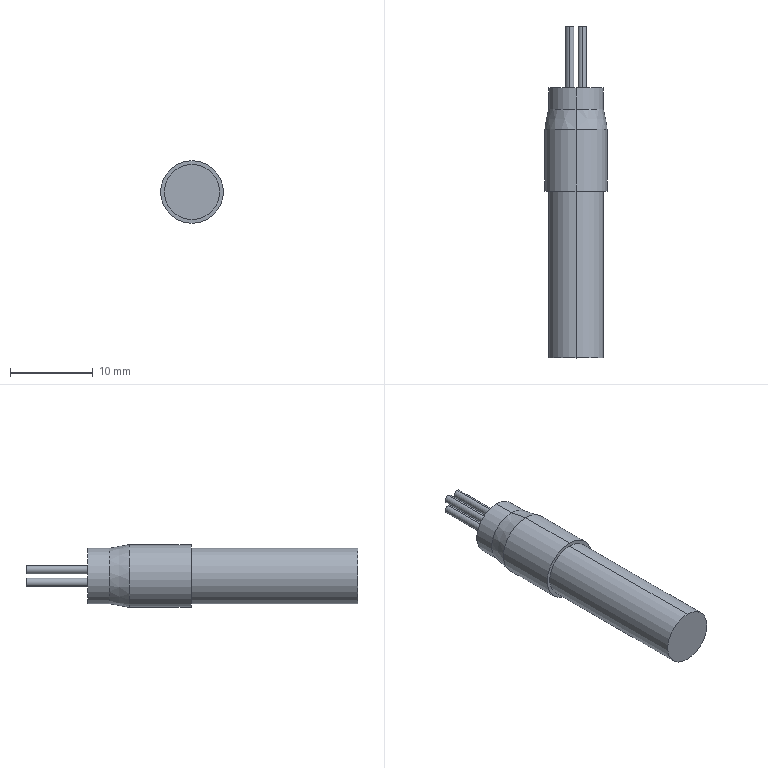Part | SolidWorks | features BaseBody 1 | 1 solid | 23 faces | box 7.6 x 40.2 x 7.6 mm | volume 1264 mm3 | cylinder 14 | plane 7 | cone 2 | commonest cylinder face diameters 1 x8 6.7 x4 7.6 x2
STEP:
#1=CARTESIAN_POINT('',(0.,72.3,3.35));
#2=VERTEX_POINT('',#1);
#3=CARTESIAN_POINT('',(0.,72.3,-3.35));
#4=VERTEX_POINT('',#3);
#5=CARTESIAN_POINT('',(0.,72.3,0.));
#6=DIRECTION('',(0.,1.,0.));
#7=DIRECTION('',(0.,0.,1.));
#8=AXIS2_PLACEMENT_3D('',#5,#6,#7);
#9=CIRCLE('',#8,3.35);
#10=EDGE_CURVE('',#2,#4,#9,.T.);
#11=ORIENTED_EDGE('',*,*,#10,.T.);
#12=CARTESIAN_POINT('',(0.,92.5,-3.35));
#13=VERTEX_POINT('',#12);
#14=CARTESIAN_POINT('',(0.,95.,-3.35));
#15=DIRECTION('',(0.,1.,0.));
#16=VECTOR('',#15,1000.);
#17=LINE('',#14,#16);
#18=EDGE_CURVE('',#4,#13,#17,.T.);
#19=ORIENTED_EDGE('',*,*,#18,.T.);
#20=CARTESIAN_POINT('',(0.,92.5,3.35));
#21=VERTEX_POINT('',#20);
#22=CARTESIAN_POINT('',(0.,92.5,0.));
#23=DIRECTION('',(0.,-1.,0.));
#24=DIRECTION('',(0.,0.,1.));
#25=AXIS2_PLACEMENT_3D('',#22,#23,#24);
#26=CIRCLE('',#25,3.35);
#27=EDGE_CURVE('',#13,#21,#26,.T.);
#28=ORIENTED_EDGE('',*,*,#27,.T.);
#29=CARTESIAN_POINT('',(0.,95.,3.35));
#30=DIRECTION('',(0.,1.,0.));
#31=VECTOR('',#30,1000.);
#32=LINE('',#29,#31);
#33=EDGE_CURVE('',#2,#21,#32,.T.);
#34=ORIENTED_EDGE('',*,*,#33,.F.);
#35=EDGE_LOOP('',(#11,#19,#28,#34));
#36=FACE_OUTER_BOUND('',#35,.T.);
#37=CARTESIAN_POINT('',(0.,95.,0.));
#38=DIRECTION('',(0.,1.,0.));
#39=DIRECTION('',(0.,0.,1.));
#40=AXIS2_PLACEMENT_3D('',#37,#38,#39);
#41=CYLINDRICAL_SURFACE('',#40,3.35);
#42=ADVANCED_FACE('',(#36),#41,.T.);
#43=CARTESIAN_POINT('',(0.,92.5,3.8));
#44=VERTEX_POINT('',#43);
#45=CARTESIAN_POINT('',(0.,92.5,-3.8));
#46=VERTEX_POINT('',#45);
#47=CARTESIAN_POINT('',(0.,92.5,0.));
#48=DIRECTION('',(0.,1.,0.));
#49=DIRECTION('',(0.,0.,1.));
#50=AXIS2_PLACEMENT_3D('',#47,#48,#49);
#51=CIRCLE('',#50,3.8);
#52=EDGE_CURVE('',#44,#46,#51,.T.);
#53=ORIENTED_EDGE('',*,*,#52,.T.);
#54=CARTESIAN_POINT('',(0.,100.,-3.8));
#55=VERTEX_POINT('',#54);
#56=CARTESIAN_POINT('',(0.,92.5,-3.8));
#57=DIRECTION('',(0.,1.,0.));
#58=VECTOR('',#57,1000.);
#59=LINE('',#56,#58);
#60=EDGE_CURVE('',#46,#55,#59,.T.);
#61=ORIENTED_EDGE('',*,*,#60,.T.);
#62=CARTESIAN_POINT('',(0.,100.,3.8));
#63=VERTEX_POINT('',#62);
#64=CARTESIAN_POINT('',(0.,100.,0.));
#65=DIRECTION('',(0.,-1.,0.));
#66=DIRECTION('',(0.,0.,1.));
#67=AXIS2_PLACEMENT_3D('',#64,#65,#66);
#68=CIRCLE('',#67,3.8);
#69=EDGE_CURVE('',#55,#63,#68,.T.);
#70=ORIENTED_EDGE('',*,*,#69,.T.);
#71=CARTESIAN_POINT('',(0.,92.5,3.8));
#72=DIRECTION('',(0.,1.,0.));
#73=VECTOR('',#72,1000.);
#74=LINE('',#71,#73);
#75=EDGE_CURVE('',#44,#63,#74,.T.);
#76=ORIENTED_EDGE('',*,*,#75,.F.);
#77=EDGE_LOOP('',(#53,#61,#70,#76));
#78=FACE_OUTER_BOUND('',#77,.T.);
#79=CARTESIAN_POINT('',(0.,92.5,0.));
#80=DIRECTION('',(0.,1.,0.));
#81=DIRECTION('',(0.,0.,1.));
#82=AXIS2_PLACEMENT_3D('',#79,#80,#81);
#83=CYLINDRICAL_SURFACE('',#82,3.8);
#84=ADVANCED_FACE('',(#78),#83,.T.);
#85=CARTESIAN_POINT('',(0.,102.426,-3.35));
#86=VERTEX_POINT('',#85);
#87=CARTESIAN_POINT('',(0.,102.426,3.35));
#88=VERTEX_POINT('',#87);
#89=CARTESIAN_POINT('',(0.,102.426,0.));
#90=DIRECTION('',(0.,-1.,0.));
#91=DIRECTION('',(0.,0.,-1.));
#92=AXIS2_PLACEMENT_3D('',#89,#90,#91);
#93=CIRCLE('',#92,3.35);
#94=EDGE_CURVE('',#86,#88,#93,.T.);
#95=ORIENTED_EDGE('',*,*,#94,.T.);
#96=CARTESIAN_POINT('',(0.,100.,3.8));
#97=DIRECTION('',(0.,-0.9832,0.1824));
#98=VECTOR('',#97,1000.);
#99=LINE('',#96,#98);
#100=EDGE_CURVE('',#88,#63,#99,.T.);
#101=ORIENTED_EDGE('',*,*,#100,.T.);
#102=ORIENTED_EDGE('',*,*,#69,.F.);
#103=CARTESIAN_POINT('',(0.,100.,-3.8));
#104=DIRECTION('',(0.,-0.9832,-0.1824));
#105=VECTOR('',#104,1000.);
#106=LINE('',#103,#105);
#107=EDGE_CURVE('',#86,#55,#106,.T.);
#108=ORIENTED_EDGE('',*,*,#107,.F.);
#109=EDGE_LOOP('',(#95,#101,#102,#108));
#110=FACE_OUTER_BOUND('',#109,.T.);
#111=CARTESIAN_POINT('',(0.,100.,0.));
#112=DIRECTION('',(0.,-1.,0.));
#113=DIRECTION('',(0.,0.,-1.));
#114=AXIS2_PLACEMENT_3D('',#111,#112,#113);
#115=CONICAL_SURFACE('',#114,3.8,0.1834);
#116=ADVANCED_FACE('',(#110),#115,.T.);
#117=ORIENTED_EDGE('',*,*,#94,.F.);
#118=CARTESIAN_POINT('',(0.,105.,-3.35));
#119=VERTEX_POINT('',#118);
#120=CARTESIAN_POINT('',(0.,92.5,-3.35));
#121=DIRECTION('',(0.,1.,0.));
#122=VECTOR('',#121,1000.);
#123=LINE('',#120,#122);
#124=EDGE_CURVE('',#86,#119,#123,.T.);
#125=ORIENTED_EDGE('',*,*,#124,.T.);
#126=CARTESIAN_POINT('',(0.,105.,3.35));
#127=VERTEX_POINT('',#126);
#128=CARTESIAN_POINT('',(0.,105.,0.));
#129=DIRECTION('',(0.,-1.,0.));
#130=DIRECTION('',(0.,0.,1.));
#131=AXIS2_PLACEMENT_3D('',#128,#129,#130);
#132=CIRCLE('',#131,3.35);
#133=EDGE_CURVE('',#119,#127,#132,.T.);
#134=ORIENTED_EDGE('',*,*,#133,.T.);
#135=CARTESIAN_POINT('',(0.,92.5,3.35));
#136=DIRECTION('',(0.,1.,0.));
#137=VECTOR('',#136,1000.);
#138=LINE('',#135,#137);
#139=EDGE_CURVE('',#88,#127,#138,.T.);
#140=ORIENTED_EDGE('',*,*,#139,.F.);
#141=EDGE_LOOP('',(#117,#125,#134,#140));
#142=FACE_OUTER_BOUND('',#141,.T.);
#143=CARTESIAN_POINT('',(0.,92.5,0.));
#144=DIRECTION('',(0.,1.,0.));
#145=DIRECTION('',(0.,0.,1.));
#146=AXIS2_PLACEMENT_3D('',#143,#144,#145);
#147=CYLINDRICAL_SURFACE('',#146,3.35);
#148=ADVANCED_FACE('',(#142),#147,.T.);
#149=CARTESIAN_POINT('',(0.75,105.,-0.25));
#150=VERTEX_POINT('',#149);
#151=CARTESIAN_POINT('',(0.75,105.,-1.25));
#152=VERTEX_POINT('',#151);
#153=CARTESIAN_POINT('',(0.75,105.,-0.75));
#154=DIRECTION('',(0.,1.,0.));
#155=DIRECTION('',(0.,0.,1.));
#156=AXIS2_PLACEMENT_3D('',#153,#154,#155);
#157=CIRCLE('',#156,0.5);
#158=EDGE_CURVE('',#150,#152,#157,.T.);
#159=ORIENTED_EDGE('',*,*,#158,.T.);
#160=CARTESIAN_POINT('',(0.75,112.5,-1.25));
#161=VERTEX_POINT('',#160);
#162=CARTESIAN_POINT('',(0.75,112.5,-1.25));
#163=DIRECTION('',(0.,1.,0.));
#164=VECTOR('',#163,1000.);
#165=LINE('',#162,#164);
#166=EDGE_CURVE('',#152,#161,#165,.T.);
#167=ORIENTED_EDGE('',*,*,#166,.T.);
#168=CARTESIAN_POINT('',(0.75,112.5,-0.25));
#169=VERTEX_POINT('',#168);
#170=CARTESIAN_POINT('',(0.75,112.5,-0.75));
#171=DIRECTION('',(0.,-1.,0.));
#172=DIRECTION('',(0.,0.,1.));
#173=AXIS2_PLACEMENT_3D('',#170,#171,#172);
#174=CIRCLE('',#173,0.5);
#175=EDGE_CURVE('',#161,#169,#174,.T.);
#176=ORIENTED_EDGE('',*,*,#175,.T.);
#177=CARTESIAN_POINT('',(0.75,112.5,-0.25));
#178=DIRECTION('',(0.,1.,0.));
#179=VECTOR('',#178,1000.);
#180=LINE('',#177,#179);
#181=EDGE_CURVE('',#150,#169,#180,.T.);
#182=ORIENTED_EDGE('',*,*,#181,.F.);
#183=EDGE_LOOP('',(#159,#167,#176,#182));
#184=FACE_OUTER_BOUND('',#183,.T.);
#185=CARTESIAN_POINT('',(0.75,112.5,-0.75));
#186=DIRECTION('',(0.,1.,0.));
#187=DIRECTION('',(0.,0.,1.));
#188=AXIS2_PLACEMENT_3D('',#185,#186,#187);
#189=CYLINDRICAL_SURFACE('',#188,0.5);
#190=ADVANCED_FACE('',(#184),#189,.T.);
#191=CARTESIAN_POINT('',(-0.75,105.,-0.25));
#192=VERTEX_POINT('',#191);
#193=CARTESIAN_POINT('',(-0.75,105.,-1.25));
#194=VERTEX_POINT('',#193);
#195=CARTESIAN_POINT('',(-0.75,105.,-0.75));
#196=DIRECTION('',(0.,1.,0.));
#197=DIRECTION('',(0.,0.,1.));
#198=AXIS2_PLACEMENT_3D('',#195,#196,#197);
#199=CIRCLE('',#198,0.5);
#200=EDGE_CURVE('',#192,#194,#199,.T.);
#201=ORIENTED_EDGE('',*,*,#200,.T.);
#202=CARTESIAN_POINT('',(-0.75,112.5,-1.25));
#203=VERTEX_POINT('',#202);
#204=CARTESIAN_POINT('',(-0.75,112.5,-1.25));
#205=DIRECTION('',(0.,1.,0.));
#206=VECTOR('',#205,1000.);
#207=LINE('',#204,#206);
#208=EDGE_CURVE('',#194,#203,#207,.T.);
#209=ORIENTED_EDGE('',*,*,#208,.T.);
#210=CARTESIAN_POINT('',(-0.75,112.5,-0.25));
#211=VERTEX_POINT('',#210);
#212=CARTESIAN_POINT('',(-0.75,112.5,-0.75));
#213=DIRECTION('',(0.,-1.,0.));
#214=DIRECTION('',(0.,0.,1.));
#215=AXIS2_PLACEMENT_3D('',#212,#213,#214);
#216=CIRCLE('',#215,0.5);
#217=EDGE_CURVE('',#203,#211,#216,.T.);
#218=ORIENTED_EDGE('',*,*,#217,.T.);
#219=CARTESIAN_POINT('',(-0.75,112.5,-0.25));
#220=DIRECTION('',(0.,1.,0.));
#221=VECTOR('',#220,1000.);
#222=LINE('',#219,#221);
#223=EDGE_CURVE('',#192,#211,#222,.T.);
#224=ORIENTED_EDGE('',*,*,#223,.F.);
#225=EDGE_LOOP('',(#201,#209,#218,#224));
#226=FACE_OUTER_BOUND('',#225,.T.);
#227=CARTESIAN_POINT('',(-0.75,112.5,-0.75));
#228=DIRECTION('',(0.,1.,0.));
#229=DIRECTION('',(0.,0.,1.));
#230=AXIS2_PLACEMENT_3D('',#227,#228,#229);
#231=CYLINDRICAL_SURFACE('',#230,0.5);
#232=ADVANCED_FACE('',(#226),#231,.T.);
#233=CARTESIAN_POINT('',(-0.75,105.,1.25));
#234=VERTEX_POINT('',#233);
#235=CARTESIAN_POINT('',(-0.75,105.,0.25));
#236=VERTEX_POINT('',#235);
#237=CARTESIAN_POINT('',(-0.75,105.,0.75));
#238=DIRECTION('',(0.,1.,0.));
#239=DIRECTION('',(0.,0.,1.));
#240=AXIS2_PLACEMENT_3D('',#237,#238,#239);
#241=CIRCLE('',#240,0.5);
#242=EDGE_CURVE('',#234,#236,#241,.T.);
#243=ORIENTED_EDGE('',*,*,#242,.T.);
#244=CARTESIAN_POINT('',(-0.75,112.5,0.25));
#245=VERTEX_POINT('',#244);
#246=CARTESIAN_POINT('',(-0.75,112.5,0.25));
#247=DIRECTION('',(0.,1.,0.));
#248=VECTOR('',#247,1000.);
#249=LINE('',#246,#248);
#250=EDGE_CURVE('',#236,#245,#249,.T.);
#251=ORIENTED_EDGE('',*,*,#250,.T.);
#252=CARTESIAN_POINT('',(-0.75,112.5,1.25));
#253=VERTEX_POINT('',#252);
#254=CARTESIAN_POINT('',(-0.75,112.5,0.75));
#255=DIRECTION('',(0.,-1.,0.));
#256=DIRECTION('',(0.,0.,1.));
#257=AXIS2_PLACEMENT_3D('',#254,#255,#256);
#258=CIRCLE('',#257,0.5);
#259=EDGE_CURVE('',#245,#253,#258,.T.);
#260=ORIENTED_EDGE('',*,*,#259,.T.);
#261=CARTESIAN_POINT('',(-0.75,112.5,1.25));
#262=DIRECTION('',(0.,1.,0.));
#263=VECTOR('',#262,1000.);
#264=LINE('',#261,#263);
#265=EDGE_CURVE('',#234,#253,#264,.T.);
#266=ORIENTED_EDGE('',*,*,#265,.F.);
#267=EDGE_LOOP('',(#243,#251,#260,#266));
#268=FACE_OUTER_BOUND('',#267,.T.);
#269=CARTESIAN_POINT('',(-0.75,112.5,0.75));
#270=DIRECTION('',(0.,1.,0.));
#271=DIRECTION('',(0.,0.,1.));
#272=AXIS2_PLACEMENT_3D('',#269,#270,#271);
#273=CYLINDRICAL_SURFACE('',#272,0.5);
#274=ADVANCED_FACE('',(#268),#273,.T.);
#275=CARTESIAN_POINT('',(0.75,105.,1.25));
#276=VERTEX_POINT('',#275);
#277=CARTESIAN_POINT('',(0.75,105.,0.25));
#278=VERTEX_POINT('',#277);
#279=CARTESIAN_POINT('',(0.75,105.,0.75));
#280=DIRECTION('',(0.,1.,0.));
#281=DIRECTION('',(0.,0.,1.));
#282=AXIS2_PLACEMENT_3D('',#279,#280,#281);
#283=CIRCLE('',#282,0.5);
#284=EDGE_CURVE('',#276,#278,#283,.T.);
#285=ORIENTED_EDGE('',*,*,#284,.T.);
#286=CARTESIAN_POINT('',(0.75,112.5,0.25));
#287=VERTEX_POINT('',#286);
#288=CARTESIAN_POINT('',(0.75,112.5,0.25));
#289=DIRECTION('',(0.,1.,0.));
#290=VECTOR('',#289,1000.);
#291=LINE('',#288,#290);
#292=EDGE_CURVE('',#278,#287,#291,.T.);
#293=ORIENTED_EDGE('',*,*,#292,.T.);
#294=CARTESIAN_POINT('',(0.75,112.5,1.25));
#295=VERTEX_POINT('',#294);
#296=CARTESIAN_POINT('',(0.75,112.5,0.75));
#297=DIRECTION('',(0.,-1.,0.));
#298=DIRECTION('',(0.,0.,1.));
#299=AXIS2_PLACEMENT_3D('',#296,#297,#298);
#300=CIRCLE('',#299,0.5);
#301=EDGE_CURVE('',#287,#295,#300,.T.);
#302=ORIENTED_EDGE('',*,*,#301,.T.);
#303=CARTESIAN_POINT('',(0.75,112.5,1.25));
#304=DIRECTION('',(0.,1.,0.));
#305=VECTOR('',#304,1000.);
#306=LINE('',#303,#305);
#307=EDGE_CURVE('',#276,#295,#306,.T.);
#308=ORIENTED_EDGE('',*,*,#307,.F.);
#309=EDGE_LOOP('',(#285,#293,#302,#308));
#310=FACE_OUTER_BOUND('',#309,.T.);
#311=CARTESIAN_POINT('',(0.75,112.5,0.75));
#312=DIRECTION('',(0.,1.,0.));
#313=DIRECTION('',(0.,0.,1.));
#314=AXIS2_PLACEMENT_3D('',#311,#312,#313);
#315=CYLINDRICAL_SURFACE('',#314,0.5);
#316=ADVANCED_FACE('',(#310),#315,.T.);
#317=ORIENTED_EDGE('',*,*,#18,.F.);
#318=CARTESIAN_POINT('',(0.,72.3,0.));
#319=DIRECTION('',(0.,1.,0.));
#320=DIRECTION('',(0.,0.,1.));
#321=AXIS2_PLACEMENT_3D('',#318,#319,#320);
#322=CIRCLE('',#321,3.35);
#323=EDGE_CURVE('',#4,#2,#322,.T.);
#324=ORIENTED_EDGE('',*,*,#323,.T.);
#325=ORIENTED_EDGE('',*,*,#33,.T.);
#326=CARTESIAN_POINT('',(0.,92.5,0.));
#327=DIRECTION('',(0.,-1.,0.));
#328=DIRECTION('',(0.,0.,1.));
#329=AXIS2_PLACEMENT_3D('',#326,#327,#328);
#330=CIRCLE('',#329,3.35);
#331=EDGE_CURVE('',#21,#13,#330,.T.);
#332=ORIENTED_EDGE('',*,*,#331,.T.);
#333=EDGE_LOOP('',(#317,#324,#325,#332));
#334=FACE_OUTER_BOUND('',#333,.T.);
#335=CARTESIAN_POINT('',(0.,95.,0.));
#336=DIRECTION('',(0.,1.,0.));
#337=DIRECTION('',(0.,0.,1.));
#338=AXIS2_PLACEMENT_3D('',#335,#336,#337);
#339=CYLINDRICAL_SURFACE('',#338,3.35);
#340=ADVANCED_FACE('',(#334),#339,.T.);
#341=ORIENTED_EDGE('',*,*,#52,.F.);
#342=CARTESIAN_POINT('',(0.,92.5,0.));
#343=DIRECTION('',(0.,1.,0.));
#344=DIRECTION('',(0.,0.,1.));
#345=AXIS2_PLACEMENT_3D('',#342,#343,#344);
#346=CIRCLE('',#345,3.8);
#347=EDGE_CURVE('',#46,#44,#346,.T.);
#348=ORIENTED_EDGE('',*,*,#347,.F.);
#349=EDGE_LOOP('',(#341,#348));
#350=FACE_OUTER_BOUND('',#349,.T.);
#351=ORIENTED_EDGE('',*,*,#331,.F.);
#352=ORIENTED_EDGE('',*,*,#27,.F.);
#353=EDGE_LOOP('',(#351,#352));
#354=FACE_BOUND('',#353,.T.);
#355=CARTESIAN_POINT('',(3.8,92.5,0.));
#356=DIRECTION('',(0.,1.,0.));
#357=DIRECTION('',(0.,0.,1.));
#358=AXIS2_PLACEMENT_3D('',#355,#356,#357);
#359=PLANE('',#358);
#360=ADVANCED_FACE('',(#350,#354),#359,.F.);
#361=ORIENTED_EDGE('',*,*,#10,.F.);
#362=ORIENTED_EDGE('',*,*,#323,.F.);
#363=EDGE_LOOP('',(#361,#362));
#364=FACE_OUTER_BOUND('',#363,.T.);
#365=CARTESIAN_POINT('',(0.,72.3,0.));
#366=DIRECTION('',(0.,1.,0.));
#367=DIRECTION('',(0.,0.,1.));
#368=AXIS2_PLACEMENT_3D('',#365,#366,#367);
#369=PLANE('',#368);
#370=ADVANCED_FACE('',(#364),#369,.F.);
#371=ORIENTED_EDGE('',*,*,#60,.F.);
#372=ORIENTED_EDGE('',*,*,#347,.T.);
#373=ORIENTED_EDGE('',*,*,#75,.T.);
#374=CARTESIAN_POINT('',(0.,100.,0.));
#375=DIRECTION('',(0.,-1.,0.));
#376=DIRECTION('',(0.,0.,1.));
#377=AXIS2_PLACEMENT_3D('',#374,#375,#376);
#378=CIRCLE('',#377,3.8);
#379=EDGE_CURVE('',#63,#55,#378,.T.);
#380=ORIENTED_EDGE('',*,*,#379,.T.);
#381=EDGE_LOOP('',(#371,#372,#373,#380));
#382=FACE_OUTER_BOUND('',#381,.T.);
#383=CARTESIAN_POINT('',(0.,92.5,0.));
#384=DIRECTION('',(0.,1.,0.));
#385=DIRECTION('',(0.,0.,1.));
#386=AXIS2_PLACEMENT_3D('',#383,#384,#385);
#387=CYLINDRICAL_SURFACE('',#386,3.8);
#388=ADVANCED_FACE('',(#382),#387,.T.);
#389=ORIENTED_EDGE('',*,*,#100,.F.);
#390=CARTESIAN_POINT('',(0.,102.426,0.));
#391=DIRECTION('',(0.,-1.,0.));
#392=DIRECTION('',(0.,0.,-1.));
#393=AXIS2_PLACEMENT_3D('',#390,#391,#392);
#394=CIRCLE('',#393,3.35);
#395=EDGE_CURVE('',#88,#86,#394,.T.);
#396=ORIENTED_EDGE('',*,*,#395,.T.);
#397=ORIENTED_EDGE('',*,*,#107,.T.);
#398=ORIENTED_EDGE('',*,*,#379,.F.);
#399=EDGE_LOOP('',(#389,#396,#397,#398));
#400=FACE_OUTER_BOUND('',#399,.T.);
#401=CARTESIAN_POINT('',(0.,100.,0.));
#402=DIRECTION('',(0.,-1.,0.));
#403=DIRECTION('',(0.,0.,-1.));
#404=AXIS2_PLACEMENT_3D('',#401,#402,#403);
#405=CONICAL_SURFACE('',#404,3.8,0.1834);
#406=ADVANCED_FACE('',(#400),#405,.T.);
#407=ORIENTED_EDGE('',*,*,#124,.F.);
#408=ORIENTED_EDGE('',*,*,#395,.F.);
#409=ORIENTED_EDGE('',*,*,#139,.T.);
#410=CARTESIAN_POINT('',(0.,105.,0.));
#411=DIRECTION('',(0.,-1.,0.));
#412=DIRECTION('',(0.,0.,1.));
#413=AXIS2_PLACEMENT_3D('',#410,#411,#412);
#414=CIRCLE('',#413,3.35);
#415=EDGE_CURVE('',#127,#119,#414,.T.);
#416=ORIENTED_EDGE('',*,*,#415,.T.);
#417=EDGE_LOOP('',(#407,#408,#409,#416));
#418=FACE_OUTER_BOUND('',#417,.T.);
#419=CARTESIAN_POINT('',(0.,92.5,0.));
#420=DIRECTION('',(0.,1.,0.));
#421=DIRECTION('',(0.,0.,1.));
#422=AXIS2_PLACEMENT_3D('',#419,#420,#421);
#423=CYLINDRICAL_SURFACE('',#422,3.35);
#424=ADVANCED_FACE('',(#418),#423,.T.);
#425=ORIENTED_EDGE('',*,*,#158,.F.);
#426=CARTESIAN_POINT('',(0.75,105.,-0.75));
#427=DIRECTION('',(0.,1.,0.));
#428=DIRECTION('',(0.,0.,1.));
#429=AXIS2_PLACEMENT_3D('',#426,#427,#428);
#430=CIRCLE('',#429,0.5);
#431=EDGE_CURVE('',#152,#150,#430,.T.);
#432=ORIENTED_EDGE('',*,*,#431,.F.);
#433=EDGE_LOOP('',(#425,#432));
#434=FACE_BOUND('',#433,.T.);
#435=ORIENTED_EDGE('',*,*,#200,.F.);
#436=CARTESIAN_POINT('',(-0.75,105.,-0.75));
#437=DIRECTION('',(0.,1.,0.));
#438=DIRECTION('',(0.,0.,1.));
#439=AXIS2_PLACEMENT_3D('',#436,#437,#438);
#440=CIRCLE('',#439,0.5);
#441=EDGE_CURVE('',#194,#192,#440,.T.);
#442=ORIENTED_EDGE('',*,*,#441,.F.);
#443=EDGE_LOOP('',(#435,#442));
#444=FACE_BOUND('',#443,.T.);
#445=ORIENTED_EDGE('',*,*,#242,.F.);
#446=CARTESIAN_POINT('',(-0.75,105.,0.75));
#447=DIRECTION('',(0.,1.,0.));
#448=DIRECTION('',(0.,0.,1.));
#449=AXIS2_PLACEMENT_3D('',#446,#447,#448);
#450=CIRCLE('',#449,0.5);
#451=EDGE_CURVE('',#236,#234,#450,.T.);
#452=ORIENTED_EDGE('',*,*,#451,.F.);
#453=EDGE_LOOP('',(#445,#452));
#454=FACE_BOUND('',#453,.T.);
#455=ORIENTED_EDGE('',*,*,#284,.F.);
#456=CARTESIAN_POINT('',(0.75,105.,0.75));
#457=DIRECTION('',(0.,1.,0.));
#458=DIRECTION('',(0.,0.,1.));
#459=AXIS2_PLACEMENT_3D('',#456,#457,#458);
#460=CIRCLE('',#459,0.5);
#461=EDGE_CURVE('',#278,#276,#460,.T.);
#462=ORIENTED_EDGE('',*,*,#461,.F.);
#463=EDGE_LOOP('',(#455,#462));
#464=FACE_BOUND('',#463,.T.);
#465=ORIENTED_EDGE('',*,*,#415,.F.);
#466=ORIENTED_EDGE('',*,*,#133,.F.);
#467=EDGE_LOOP('',(#465,#466));
#468=FACE_OUTER_BOUND('',#467,.T.);
#469=CARTESIAN_POINT('',(0.,105.,0.));
#470=DIRECTION('',(0.,-1.,0.));
#471=DIRECTION('',(0.,0.,-1.));
#472=AXIS2_PLACEMENT_3D('',#469,#470,#471);
#473=PLANE('',#472);
#474=ADVANCED_FACE('',(#434,#444,#454,#464,#468),#473,.F.);
#475=ORIENTED_EDGE('',*,*,#166,.F.);
#476=ORIENTED_EDGE('',*,*,#431,.T.);
#477=ORIENTED_EDGE('',*,*,#181,.T.);
#478=CARTESIAN_POINT('',(0.75,112.5,-0.75));
#479=DIRECTION('',(0.,-1.,0.));
#480=DIRECTION('',(0.,0.,1.));
#481=AXIS2_PLACEMENT_3D('',#478,#479,#480);
#482=CIRCLE('',#481,0.5);
#483=EDGE_CURVE('',#169,#161,#482,.T.);
#484=ORIENTED_EDGE('',*,*,#483,.T.);
#485=EDGE_LOOP('',(#475,#476,#477,#484));
#486=FACE_OUTER_BOUND('',#485,.T.);
#487=CARTESIAN_POINT('',(0.75,112.5,-0.75));
#488=DIRECTION('',(0.,1.,0.));
#489=DIRECTION('',(0.,0.,1.));
#490=AXIS2_PLACEMENT_3D('',#487,#488,#489);
#491=CYLINDRICAL_SURFACE('',#490,0.5);
#492=ADVANCED_FACE('',(#486),#491,.T.);
#493=ORIENTED_EDGE('',*,*,#208,.F.);
#494=ORIENTED_EDGE('',*,*,#441,.T.);
#495=ORIENTED_EDGE('',*,*,#223,.T.);
#496=CARTESIAN_POINT('',(-0.75,112.5,-0.75));
#497=DIRECTION('',(0.,-1.,0.));
#498=DIRECTION('',(0.,0.,1.));
#499=AXIS2_PLACEMENT_3D('',#496,#497,#498);
#500=CIRCLE('',#499,0.5);
#501=EDGE_CURVE('',#211,#203,#500,.T.);
#502=ORIENTED_EDGE('',*,*,#501,.T.);
#503=EDGE_LOOP('',(#493,#494,#495,#502));
#504=FACE_OUTER_BOUND('',#503,.T.);
#505=CARTESIAN_POINT('',(-0.75,112.5,-0.75));
#506=DIRECTION('',(0.,1.,0.));
#507=DIRECTION('',(0.,0.,1.));
#508=AXIS2_PLACEMENT_3D('',#505,#506,#507);
#509=CYLINDRICAL_SURFACE('',#508,0.5);
#510=ADVANCED_FACE('',(#504),#509,.T.);
#511=ORIENTED_EDGE('',*,*,#250,.F.);
#512=ORIENTED_EDGE('',*,*,#451,.T.);
#513=ORIENTED_EDGE('',*,*,#265,.T.);
#514=CARTESIAN_POINT('',(-0.75,112.5,0.75));
#515=DIRECTION('',(0.,-1.,0.));
#516=DIRECTION('',(0.,0.,1.));
#517=AXIS2_PLACEMENT_3D('',#514,#515,#516);
#518=CIRCLE('',#517,0.5);
#519=EDGE_CURVE('',#253,#245,#518,.T.);
#520=ORIENTED_EDGE('',*,*,#519,.T.);
#521=EDGE_LOOP('',(#511,#512,#513,#520));
#522=FACE_OUTER_BOUND('',#521,.T.);
#523=CARTESIAN_POINT('',(-0.75,112.5,0.75));
#524=DIRECTION('',(0.,1.,0.));
#525=DIRECTION('',(0.,0.,1.));
#526=AXIS2_PLACEMENT_3D('',#523,#524,#525);
#527=CYLINDRICAL_SURFACE('',#526,0.5);
#528=ADVANCED_FACE('',(#522),#527,.T.);
#529=ORIENTED_EDGE('',*,*,#292,.F.);
#530=ORIENTED_EDGE('',*,*,#461,.T.);
#531=ORIENTED_EDGE('',*,*,#307,.T.);
#532=CARTESIAN_POINT('',(0.75,112.5,0.75));
#533=DIRECTION('',(0.,-1.,0.));
#534=DIRECTION('',(0.,0.,1.));
#535=AXIS2_PLACEMENT_3D('',#532,#533,#534);
#536=CIRCLE('',#535,0.5);
#537=EDGE_CURVE('',#295,#287,#536,.T.);
#538=ORIENTED_EDGE('',*,*,#537,.T.);
#539=EDGE_LOOP('',(#529,#530,#531,#538));
#540=FACE_OUTER_BOUND('',#539,.T.);
#541=CARTESIAN_POINT('',(0.75,112.5,0.75));
#542=DIRECTION('',(0.,1.,0.));
#543=DIRECTION('',(0.,0.,1.));
#544=AXIS2_PLACEMENT_3D('',#541,#542,#543);
#545=CYLINDRICAL_SURFACE('',#544,0.5);
#546=ADVANCED_FACE('',(#540),#545,.T.);
#547=ORIENTED_EDGE('',*,*,#483,.F.);
#548=ORIENTED_EDGE('',*,*,#175,.F.);
#549=EDGE_LOOP('',(#547,#548));
#550=FACE_OUTER_BOUND('',#549,.T.);
#551=CARTESIAN_POINT('',(0.75,112.5,-0.75));
#552=DIRECTION('',(0.,1.,0.));
#553=DIRECTION('',(0.,0.,1.));
#554=AXIS2_PLACEMENT_3D('',#551,#552,#553);
#555=PLANE('',#554);
#556=ADVANCED_FACE('',(#550),#555,.T.);
#557=ORIENTED_EDGE('',*,*,#501,.F.);
#558=ORIENTED_EDGE('',*,*,#217,.F.);
#559=EDGE_LOOP('',(#557,#558));
#560=FACE_OUTER_BOUND('',#559,.T.);
#561=CARTESIAN_POINT('',(-0.75,112.5,-0.75));
#562=DIRECTION('',(0.,1.,0.));
#563=DIRECTION('',(0.,0.,1.));
#564=AXIS2_PLACEMENT_3D('',#561,#562,#563);
#565=PLANE('',#564);
#566=ADVANCED_FACE('',(#560),#565,.T.);
#567=ORIENTED_EDGE('',*,*,#519,.F.);
#568=ORIENTED_EDGE('',*,*,#259,.F.);
#569=EDGE_LOOP('',(#567,#568));
#570=FACE_OUTER_BOUND('',#569,.T.);
#571=CARTESIAN_POINT('',(-0.75,112.5,0.75));
#572=DIRECTION('',(0.,1.,0.));
#573=DIRECTION('',(0.,0.,1.));
#574=AXIS2_PLACEMENT_3D('',#571,#572,#573);
#575=PLANE('',#574);
#576=ADVANCED_FACE('',(#570),#575,.T.);
#577=ORIENTED_EDGE('',*,*,#537,.F.);
#578=ORIENTED_EDGE('',*,*,#301,.F.);
#579=EDGE_LOOP('',(#577,#578));
#580=FACE_OUTER_BOUND('',#579,.T.);
#581=CARTESIAN_POINT('',(0.75,112.5,0.75));
#582=DIRECTION('',(0.,1.,0.));
#583=DIRECTION('',(0.,0.,1.));
#584=AXIS2_PLACEMENT_3D('',#581,#582,#583);
#585=PLANE('',#584);
#586=ADVANCED_FACE('',(#580),#585,.T.);
#587=CLOSED_SHELL('',(#42,#84,#116,#148,#190,#232,#274,#316,#340,#360,#370,#388,#406,#424,#474,#492,#510,#528,#546,#556,#566,#576,#586));
#588=MANIFOLD_SOLID_BREP('',#587);
#589=CARTESIAN_POINT('',(0.,0.,0.));
#590=DIRECTION('',(0.,0.,1.));
#591=DIRECTION('',(1.,0.,0.));
#592=AXIS2_PLACEMENT_3D('',#589,#590,#591);
#593=(LENGTH_UNIT()NAMED_UNIT(*)SI_UNIT(.MILLI.,.METRE.));
#594=UNCERTAINTY_MEASURE_WITH_UNIT(LENGTH_MEASURE(0.00001),#593,'','');
#595=(NAMED_UNIT(*)PLANE_ANGLE_UNIT()SI_UNIT($,.RADIAN.));
#596=(NAMED_UNIT(*)SI_UNIT($,.STERADIAN.)SOLID_ANGLE_UNIT());
#597=(GEOMETRIC_REPRESENTATION_CONTEXT(3)GLOBAL_UNCERTAINTY_ASSIGNED_CONTEXT((#594))GLOBAL_UNIT_ASSIGNED_CONTEXT((#593,#595,#596))REPRESENTATION_CONTEXT('',''));
#598=ADVANCED_BREP_SHAPE_REPRESENTATION('',(#588,#592),#597);